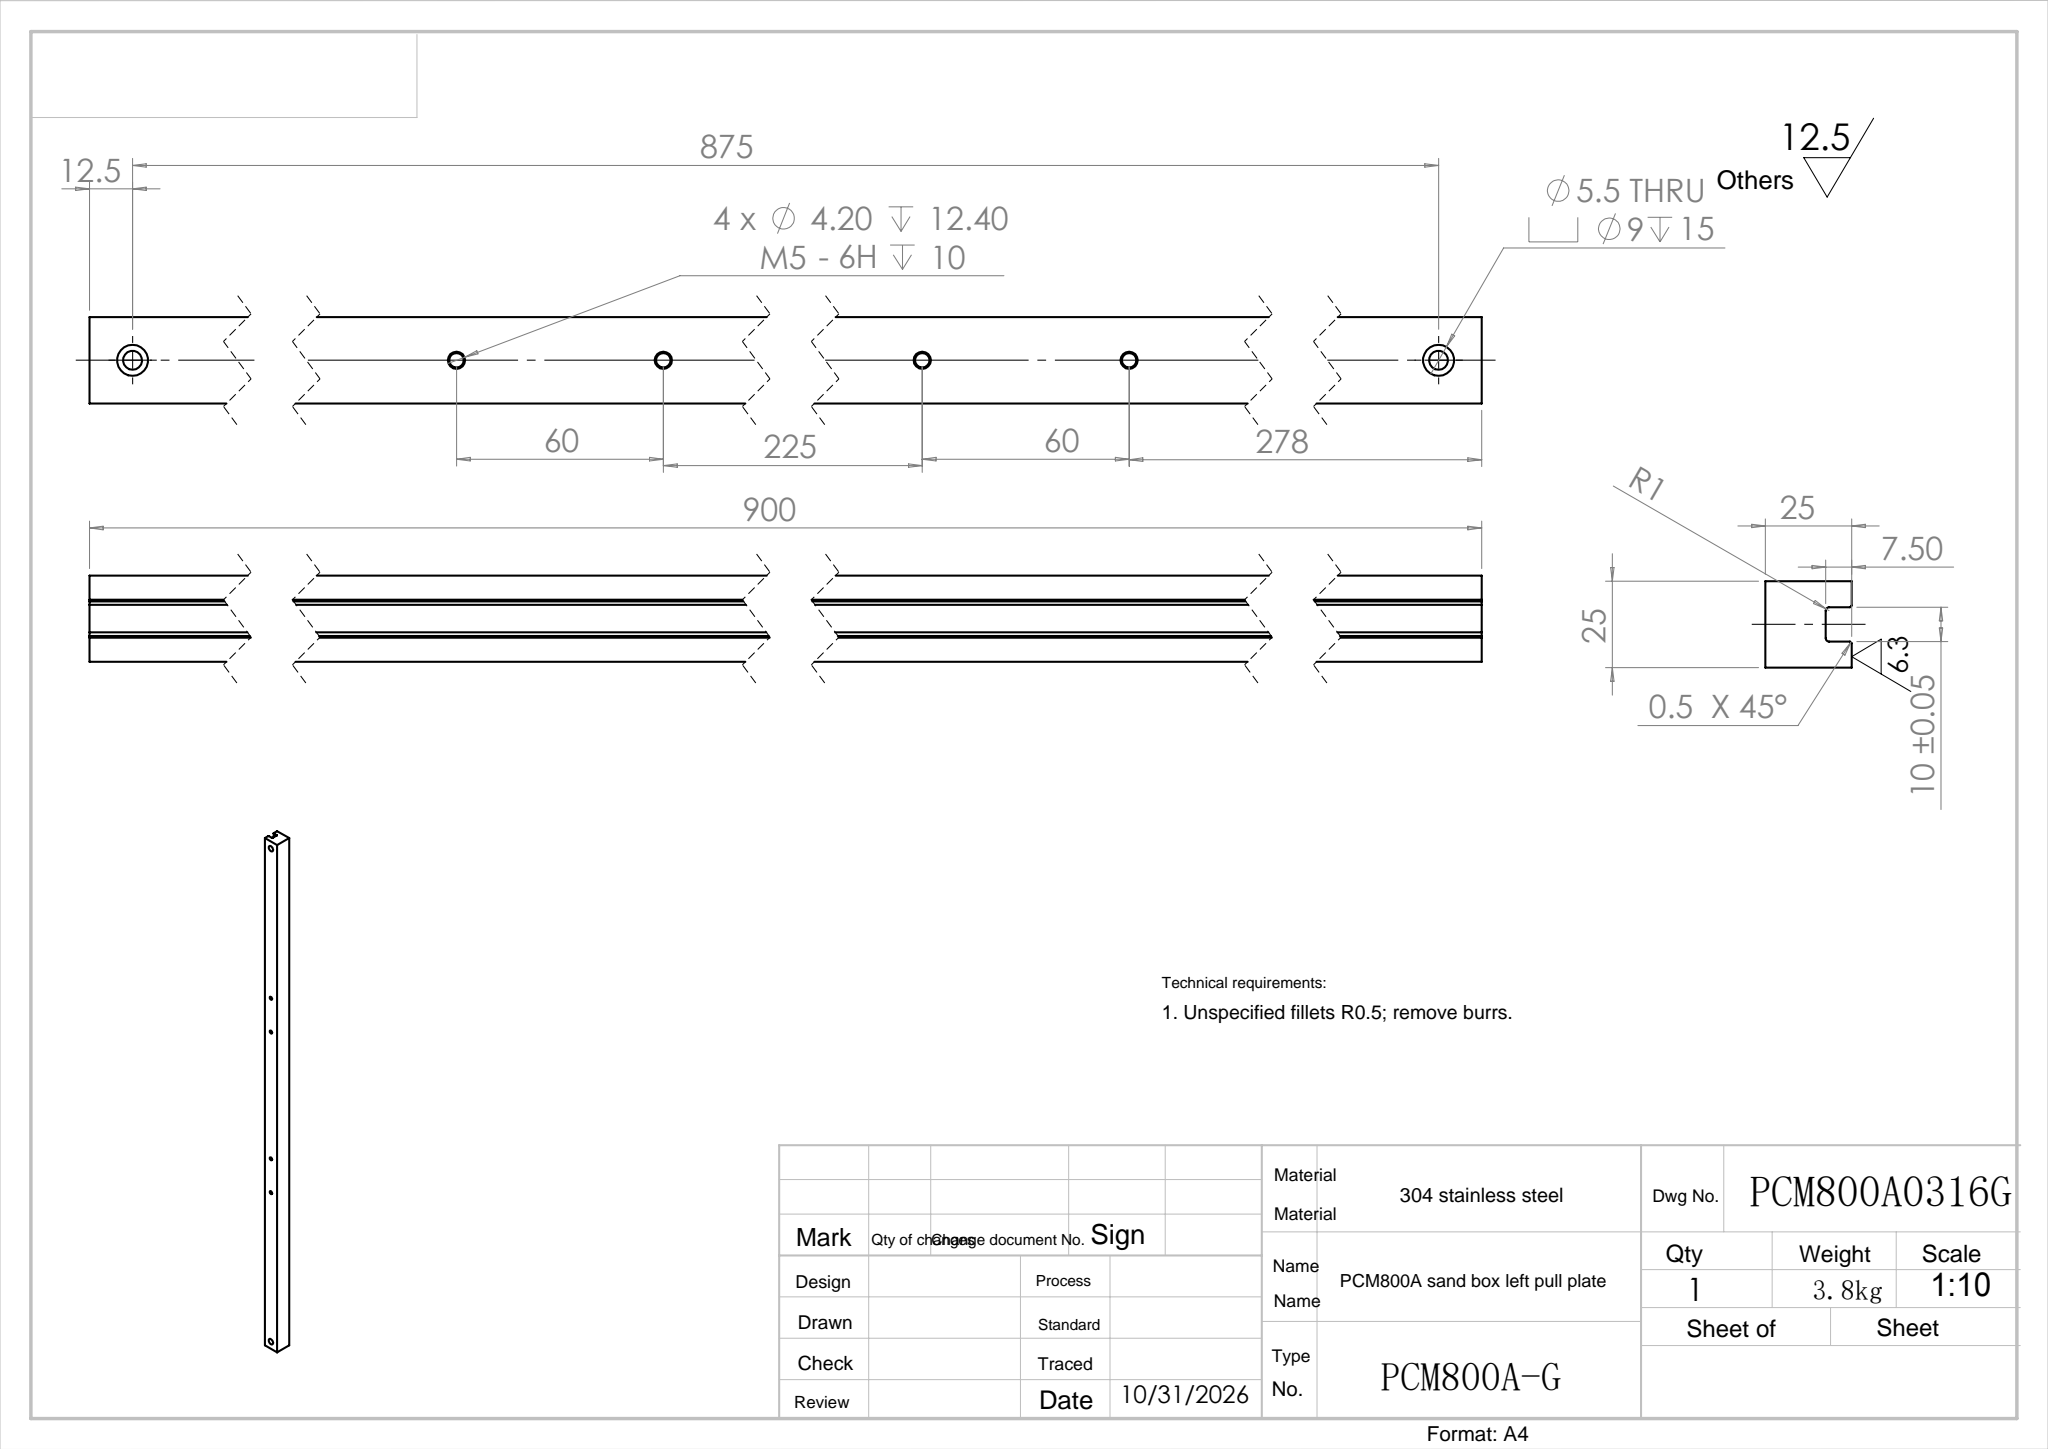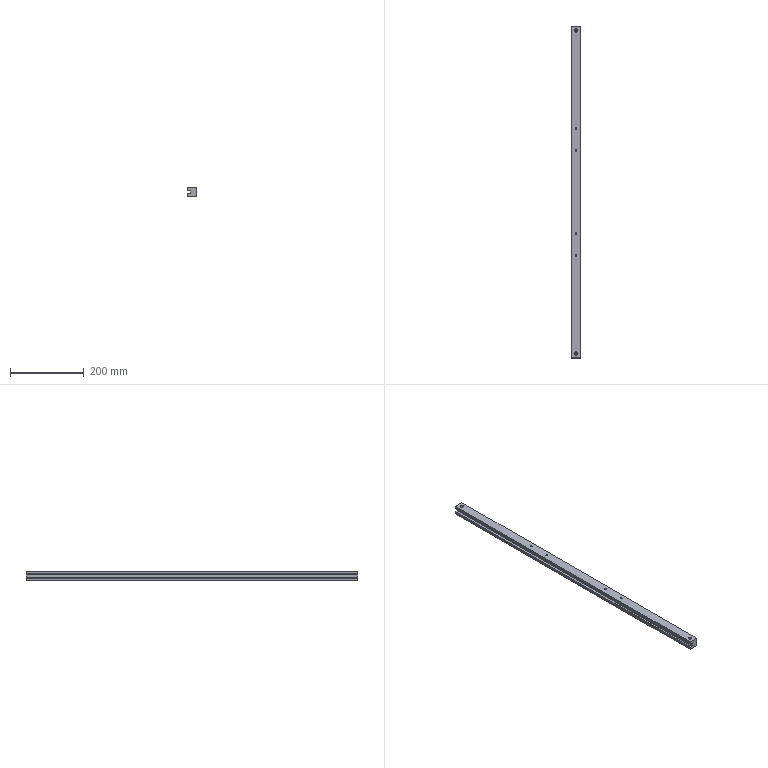Part | SolidWorks | features 3DProfileFeature 2, HoleWzd 2, Chamfer 1, Cut 1, Extrusion 1, LPattern 1 | 1 solid | 52 faces | box 25 x 900 x 25 mm | volume 491836 mm3 | cylinder 26 | plane 18 | cone 8 | commonest cylinder face diameters 4.2 x8 5 x8 5.5 x4 9 x4 2 x2